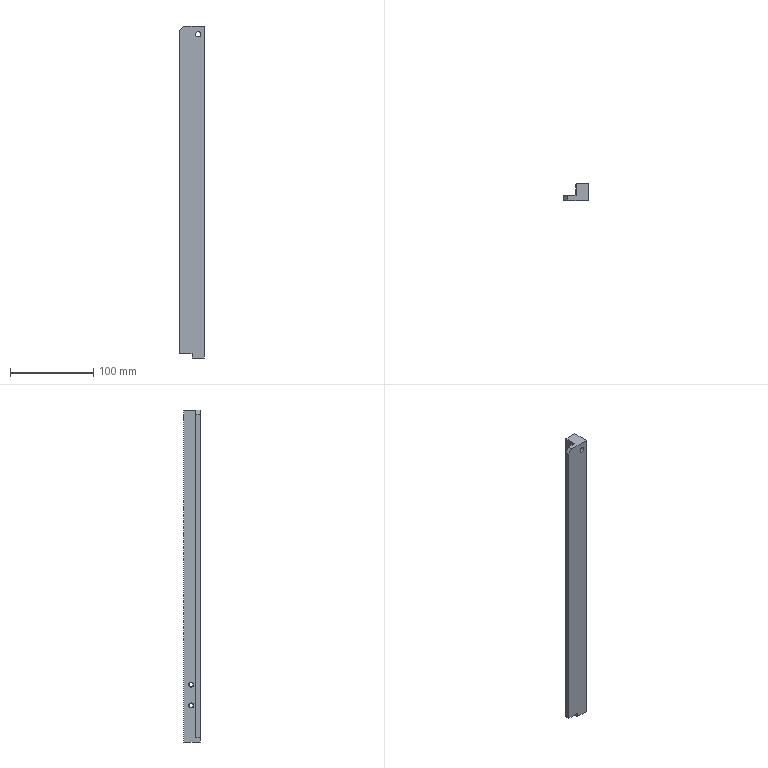Part | STEP file | Tube necking machine_id654_x_t | 1 solid | 17 faces | box 30 x 20 x 400 mm | volume 151258 mm3 | plane 10 | cone 4 | cylinder 3 | commonest cylinder face diameters 5 x2 6.5 x1
STEP:
#1=CARTESIAN_POINT('',(0.,0.,0.));
#2=DIRECTION('',(0.,0.,1.));
#3=DIRECTION('',(1.,0.,0.));
#4=AXIS2_PLACEMENT_3D('',#1,#2,#3);
#5=CARTESIAN_POINT('',(112.5,-108.,191.));
#6=VERTEX_POINT('',#5);
#7=CARTESIAN_POINT('',(97.5,-108.,191.));
#8=VERTEX_POINT('',#7);
#9=CARTESIAN_POINT('',(-10.,-108.,191.));
#10=DIRECTION('',(-1.,0.,0.));
#11=VECTOR('',#10,1.);
#12=LINE('',#9,#11);
#13=CARTESIAN_POINT('',(-10.,0.,191.));
#14=DIRECTION('',(0.,0.,1.));
#15=DIRECTION('',(-1.,0.,0.));
#16=AXIS2_PLACEMENT_3D('',#13,#14,#15);
#17=PLANE('',#16);
#18=CARTESIAN_POINT('',(0.,108.));
#19=DIRECTION('',(1.,0.));
#20=VECTOR('',#19,1.);
#21=LINE('',#18,#20);
#22=(GEOMETRIC_REPRESENTATION_CONTEXT(2)PARAMETRIC_REPRESENTATION_CONTEXT()REPRESENTATION_CONTEXT('',''));
#23=DEFINITIONAL_REPRESENTATION('',(#21),#22);
#24=PCURVE('',#17,#23);
#25=CARTESIAN_POINT('',(93.496,-108.,597.));
#26=DIRECTION('',(0.,1.,0.));
#27=DIRECTION('',(-1.,0.,0.));
#28=AXIS2_PLACEMENT_3D('',#25,#26,#27);
#29=PLANE('',#28);
#30=CARTESIAN_POINT('',(103.496,-406.));
#31=DIRECTION('',(1.,0.));
#32=VECTOR('',#31,1.);
#33=LINE('',#30,#32);
#34=(GEOMETRIC_REPRESENTATION_CONTEXT(2)PARAMETRIC_REPRESENTATION_CONTEXT()REPRESENTATION_CONTEXT('',''));
#35=DEFINITIONAL_REPRESENTATION('',(#33),#34);
#36=PCURVE('',#29,#35);
#37=SURFACE_CURVE('',#12,(#24,#36),.PCURVE_S1.);
#38=EDGE_CURVE('',#6,#8,#37,.T.);
#39=ORIENTED_EDGE('',*,*,#38,.F.);
#40=CARTESIAN_POINT('',(112.5,-128.,191.));
#41=VERTEX_POINT('',#40);
#42=CARTESIAN_POINT('',(112.5,-76.,191.));
#43=DIRECTION('',(0.,1.,0.));
#44=VECTOR('',#43,1.);
#45=LINE('',#42,#44);
#46=CARTESIAN_POINT('',(-122.5,76.));
#47=DIRECTION('',(0.,-1.));
#48=VECTOR('',#47,1.);
#49=LINE('',#46,#48);
#50=(GEOMETRIC_REPRESENTATION_CONTEXT(2)PARAMETRIC_REPRESENTATION_CONTEXT()REPRESENTATION_CONTEXT('',''));
#51=DEFINITIONAL_REPRESENTATION('',(#49),#50);
#52=PCURVE('',#17,#51);
#53=CARTESIAN_POINT('',(112.5,-76.,191.));
#54=DIRECTION('',(1.,0.,0.));
#55=DIRECTION('',(0.,-1.,0.));
#56=AXIS2_PLACEMENT_3D('',#53,#54,#55);
#57=PLANE('',#56);
#58=CARTESIAN_POINT('',(0.,0.));
#59=DIRECTION('',(-1.,0.));
#60=VECTOR('',#59,1.);
#61=LINE('',#58,#60);
#62=(GEOMETRIC_REPRESENTATION_CONTEXT(2)PARAMETRIC_REPRESENTATION_CONTEXT()REPRESENTATION_CONTEXT('',''));
#63=DEFINITIONAL_REPRESENTATION('',(#61),#62);
#64=PCURVE('',#57,#63);
#65=SURFACE_CURVE('',#45,(#52,#64),.PCURVE_S1.);
#66=EDGE_CURVE('',#41,#6,#65,.T.);
#67=ORIENTED_EDGE('',*,*,#66,.F.);
#68=CARTESIAN_POINT('',(97.5,-128.,191.));
#69=VERTEX_POINT('',#68);
#70=CARTESIAN_POINT('',(112.5,-128.,191.));
#71=DIRECTION('',(1.,0.,0.));
#72=VECTOR('',#71,1.);
#73=LINE('',#70,#72);
#74=CARTESIAN_POINT('',(-122.5,128.));
#75=DIRECTION('',(-1.,0.));
#76=VECTOR('',#75,1.);
#77=LINE('',#74,#76);
#78=(GEOMETRIC_REPRESENTATION_CONTEXT(2)PARAMETRIC_REPRESENTATION_CONTEXT()REPRESENTATION_CONTEXT('',''));
#79=DEFINITIONAL_REPRESENTATION('',(#77),#78);
#80=PCURVE('',#17,#79);
#81=CARTESIAN_POINT('',(112.5,-128.,191.));
#82=DIRECTION('',(0.,-1.,0.));
#83=DIRECTION('',(0.,0.,-1.));
#84=AXIS2_PLACEMENT_3D('',#81,#82,#83);
#85=PLANE('',#84);
#86=CARTESIAN_POINT('',(0.,0.));
#87=DIRECTION('',(0.,1.));
#88=VECTOR('',#87,1.);
#89=LINE('',#86,#88);
#90=(GEOMETRIC_REPRESENTATION_CONTEXT(2)PARAMETRIC_REPRESENTATION_CONTEXT()REPRESENTATION_CONTEXT('',''));
#91=DEFINITIONAL_REPRESENTATION('',(#89),#90);
#92=PCURVE('',#85,#91);
#93=SURFACE_CURVE('',#73,(#80,#92),.PCURVE_S1.);
#94=EDGE_CURVE('',#69,#41,#93,.T.);
#95=ORIENTED_EDGE('',*,*,#94,.F.);
#96=CARTESIAN_POINT('',(97.5,-124.5,191.));
#97=DIRECTION('',(0.,-1.,0.));
#98=VECTOR('',#97,1.);
#99=LINE('',#96,#98);
#100=CARTESIAN_POINT('',(-107.5,124.5));
#101=DIRECTION('',(0.,1.));
#102=VECTOR('',#101,1.);
#103=LINE('',#100,#102);
#104=(GEOMETRIC_REPRESENTATION_CONTEXT(2)PARAMETRIC_REPRESENTATION_CONTEXT()REPRESENTATION_CONTEXT('',''));
#105=DEFINITIONAL_REPRESENTATION('',(#103),#104);
#106=PCURVE('',#17,#105);
#107=CARTESIAN_POINT('',(97.5,-124.5,191.));
#108=DIRECTION('',(-1.,0.,0.));
#109=DIRECTION('',(0.,0.,-1.));
#110=AXIS2_PLACEMENT_3D('',#107,#108,#109);
#111=PLANE('',#110);
#112=CARTESIAN_POINT('',(0.,0.));
#113=DIRECTION('',(0.,1.));
#114=VECTOR('',#113,1.);
#115=LINE('',#112,#114);
#116=(GEOMETRIC_REPRESENTATION_CONTEXT(2)PARAMETRIC_REPRESENTATION_CONTEXT()REPRESENTATION_CONTEXT('',''));
#117=DEFINITIONAL_REPRESENTATION('',(#115),#116);
#118=PCURVE('',#111,#117);
#119=SURFACE_CURVE('',#99,(#106,#118),.PCURVE_S1.);
#120=EDGE_CURVE('',#8,#69,#119,.T.);
#121=ORIENTED_EDGE('',*,*,#120,.F.);
#122=EDGE_LOOP('',(#39,#67,#95,#121));
#123=FACE_BOUND('',#122,.T.);
#124=ADVANCED_FACE('',(#123),#17,.F.);
#125=CARTESIAN_POINT('',(112.5,-114.,235.));
#126=VERTEX_POINT('',#125);
#127=CARTESIAN_POINT('',(112.5,-117.,232.));
#128=VERTEX_POINT('',#127);
#129=CARTESIAN_POINT('',(112.5,-117.,235.));
#130=DIRECTION('',(-1.,0.,0.));
#131=DIRECTION('',(0.,1.,0.));
#132=AXIS2_PLACEMENT_3D('',#129,#130,#131);
#133=CIRCLE('',#132,3.);
#134=CARTESIAN_POINT('',(38.,-44.));
#135=CARTESIAN_POINT('',(38.,-38.804));
#136=CARTESIAN_POINT('',(42.5,-41.402));
#137=CARTESIAN_POINT('',(47.,-44.));
#138=CARTESIAN_POINT('',(42.5,-46.598));
#139=CARTESIAN_POINT('',(38.,-49.196));
#140=CARTESIAN_POINT('',(38.,-44.));
#141=(BOUNDED_CURVE()B_SPLINE_CURVE(2,(#134,#135,#136,#137,#138,#139,#140),.UNSPECIFIED.,.T.,.F.)B_SPLINE_CURVE_WITH_KNOTS((1,2,2,2,2,1),(-2.094,0.,2.094,4.189,6.283,8.378),.UNSPECIFIED.)CURVE()GEOMETRIC_REPRESENTATION_ITEM()RATIONAL_B_SPLINE_CURVE((1.,0.5,1.,0.5,1.,0.5,1.))REPRESENTATION_ITEM(''));
#142=(GEOMETRIC_REPRESENTATION_CONTEXT(2)PARAMETRIC_REPRESENTATION_CONTEXT()REPRESENTATION_CONTEXT('',''));
#143=DEFINITIONAL_REPRESENTATION('',(#141),#142);
#144=PCURVE('',#57,#143);
#145=CARTESIAN_POINT('',(112.5,-117.,235.));
#146=DIRECTION('',(1.,0.,0.));
#147=DIRECTION('',(0.,0.,-1.));
#148=AXIS2_PLACEMENT_3D('',#145,#146,#147);
#149=CONICAL_SURFACE('',#148,3.,0.7854);
#150=CARTESIAN_POINT('',(1.571,0.));
#151=DIRECTION('',(-1.,0.));
#152=VECTOR('',#151,1.);
#153=LINE('',#150,#152);
#154=(GEOMETRIC_REPRESENTATION_CONTEXT(2)PARAMETRIC_REPRESENTATION_CONTEXT()REPRESENTATION_CONTEXT('',''));
#155=DEFINITIONAL_REPRESENTATION('',(#153),#154);
#156=PCURVE('',#149,#155);
#157=SURFACE_CURVE('',#133,(#144,#156),.PCURVE_S1.);
#158=EDGE_CURVE('',#126,#128,#157,.T.);
#159=ORIENTED_EDGE('',*,*,#158,.T.);
#160=CARTESIAN_POINT('',(112.5,-117.,235.));
#161=DIRECTION('',(-1.,0.,0.));
#162=DIRECTION('',(0.,1.,0.));
#163=AXIS2_PLACEMENT_3D('',#160,#161,#162);
#164=CIRCLE('',#163,3.);
#165=CARTESIAN_POINT('',(38.,-44.));
#166=CARTESIAN_POINT('',(38.,-38.804));
#167=CARTESIAN_POINT('',(42.5,-41.402));
#168=CARTESIAN_POINT('',(47.,-44.));
#169=CARTESIAN_POINT('',(42.5,-46.598));
#170=CARTESIAN_POINT('',(38.,-49.196));
#171=CARTESIAN_POINT('',(38.,-44.));
#172=(BOUNDED_CURVE()B_SPLINE_CURVE(2,(#165,#166,#167,#168,#169,#170,#171),.UNSPECIFIED.,.T.,.F.)B_SPLINE_CURVE_WITH_KNOTS((1,2,2,2,2,1),(-2.094,0.,2.094,4.189,6.283,8.378),.UNSPECIFIED.)CURVE()GEOMETRIC_REPRESENTATION_ITEM()RATIONAL_B_SPLINE_CURVE((1.,0.5,1.,0.5,1.,0.5,1.))REPRESENTATION_ITEM(''));
#173=(GEOMETRIC_REPRESENTATION_CONTEXT(2)PARAMETRIC_REPRESENTATION_CONTEXT()REPRESENTATION_CONTEXT('',''));
#174=DEFINITIONAL_REPRESENTATION('',(#172),#173);
#175=PCURVE('',#57,#174);
#176=CARTESIAN_POINT('',(7.854,0.));
#177=DIRECTION('',(-1.,0.));
#178=VECTOR('',#177,1.);
#179=LINE('',#176,#178);
#180=(GEOMETRIC_REPRESENTATION_CONTEXT(2)PARAMETRIC_REPRESENTATION_CONTEXT()REPRESENTATION_CONTEXT('',''));
#181=DEFINITIONAL_REPRESENTATION('',(#179),#180);
#182=PCURVE('',#149,#181);
#183=SURFACE_CURVE('',#164,(#175,#182),.PCURVE_S1.);
#184=EDGE_CURVE('',#128,#126,#183,.T.);
#185=ORIENTED_EDGE('',*,*,#184,.T.);
#186=EDGE_LOOP('',(#159,#185));
#187=FACE_BOUND('',#186,.T.);
#188=CARTESIAN_POINT('',(112.5,-114.,260.));
#189=VERTEX_POINT('',#188);
#190=CARTESIAN_POINT('',(112.5,-117.,257.));
#191=VERTEX_POINT('',#190);
#192=CARTESIAN_POINT('',(112.5,-117.,260.));
#193=DIRECTION('',(-1.,0.,0.));
#194=DIRECTION('',(0.,1.,0.));
#195=AXIS2_PLACEMENT_3D('',#192,#193,#194);
#196=CIRCLE('',#195,3.);
#197=CARTESIAN_POINT('',(38.,-69.));
#198=CARTESIAN_POINT('',(38.,-63.804));
#199=CARTESIAN_POINT('',(42.5,-66.402));
#200=CARTESIAN_POINT('',(47.,-69.));
#201=CARTESIAN_POINT('',(42.5,-71.598));
#202=CARTESIAN_POINT('',(38.,-74.196));
#203=CARTESIAN_POINT('',(38.,-69.));
#204=(BOUNDED_CURVE()B_SPLINE_CURVE(2,(#197,#198,#199,#200,#201,#202,#203),.UNSPECIFIED.,.T.,.F.)B_SPLINE_CURVE_WITH_KNOTS((1,2,2,2,2,1),(-2.094,0.,2.094,4.189,6.283,8.378),.UNSPECIFIED.)CURVE()GEOMETRIC_REPRESENTATION_ITEM()RATIONAL_B_SPLINE_CURVE((1.,0.5,1.,0.5,1.,0.5,1.))REPRESENTATION_ITEM(''));
#205=(GEOMETRIC_REPRESENTATION_CONTEXT(2)PARAMETRIC_REPRESENTATION_CONTEXT()REPRESENTATION_CONTEXT('',''));
#206=DEFINITIONAL_REPRESENTATION('',(#204),#205);
#207=PCURVE('',#57,#206);
#208=CARTESIAN_POINT('',(112.5,-117.,260.));
#209=DIRECTION('',(1.,0.,0.));
#210=DIRECTION('',(0.,0.,-1.));
#211=AXIS2_PLACEMENT_3D('',#208,#209,#210);
#212=CONICAL_SURFACE('',#211,3.,0.7854);
#213=CARTESIAN_POINT('',(1.571,0.));
#214=DIRECTION('',(-1.,0.));
#215=VECTOR('',#214,1.);
#216=LINE('',#213,#215);
#217=(GEOMETRIC_REPRESENTATION_CONTEXT(2)PARAMETRIC_REPRESENTATION_CONTEXT()REPRESENTATION_CONTEXT('',''));
#218=DEFINITIONAL_REPRESENTATION('',(#216),#217);
#219=PCURVE('',#212,#218);
#220=SURFACE_CURVE('',#196,(#207,#219),.PCURVE_S1.);
#221=EDGE_CURVE('',#189,#191,#220,.T.);
#222=ORIENTED_EDGE('',*,*,#221,.T.);
#223=CARTESIAN_POINT('',(112.5,-117.,260.));
#224=DIRECTION('',(-1.,0.,0.));
#225=DIRECTION('',(0.,1.,0.));
#226=AXIS2_PLACEMENT_3D('',#223,#224,#225);
#227=CIRCLE('',#226,3.);
#228=CARTESIAN_POINT('',(38.,-69.));
#229=CARTESIAN_POINT('',(38.,-63.804));
#230=CARTESIAN_POINT('',(42.5,-66.402));
#231=CARTESIAN_POINT('',(47.,-69.));
#232=CARTESIAN_POINT('',(42.5,-71.598));
#233=CARTESIAN_POINT('',(38.,-74.196));
#234=CARTESIAN_POINT('',(38.,-69.));
#235=(BOUNDED_CURVE()B_SPLINE_CURVE(2,(#228,#229,#230,#231,#232,#233,#234),.UNSPECIFIED.,.T.,.F.)B_SPLINE_CURVE_WITH_KNOTS((1,2,2,2,2,1),(-2.094,0.,2.094,4.189,6.283,8.378),.UNSPECIFIED.)CURVE()GEOMETRIC_REPRESENTATION_ITEM()RATIONAL_B_SPLINE_CURVE((1.,0.5,1.,0.5,1.,0.5,1.))REPRESENTATION_ITEM(''));
#236=(GEOMETRIC_REPRESENTATION_CONTEXT(2)PARAMETRIC_REPRESENTATION_CONTEXT()REPRESENTATION_CONTEXT('',''));
#237=DEFINITIONAL_REPRESENTATION('',(#235),#236);
#238=PCURVE('',#57,#237);
#239=CARTESIAN_POINT('',(7.854,0.));
#240=DIRECTION('',(-1.,0.));
#241=VECTOR('',#240,1.);
#242=LINE('',#239,#241);
#243=(GEOMETRIC_REPRESENTATION_CONTEXT(2)PARAMETRIC_REPRESENTATION_CONTEXT()REPRESENTATION_CONTEXT('',''));
#244=DEFINITIONAL_REPRESENTATION('',(#242),#243);
#245=PCURVE('',#212,#244);
#246=SURFACE_CURVE('',#227,(#238,#245),.PCURVE_S1.);
#247=EDGE_CURVE('',#191,#189,#246,.T.);
#248=ORIENTED_EDGE('',*,*,#247,.T.);
#249=EDGE_LOOP('',(#222,#248));
#250=FACE_BOUND('',#249,.T.);
#251=ORIENTED_EDGE('',*,*,#66,.T.);
#252=CARTESIAN_POINT('',(112.5,-108.,591.));
#253=VERTEX_POINT('',#252);
#254=CARTESIAN_POINT('',(112.5,-108.,191.));
#255=DIRECTION('',(0.,0.,1.));
#256=VECTOR('',#255,1.);
#257=LINE('',#254,#256);
#258=CARTESIAN_POINT('',(32.,0.));
#259=DIRECTION('',(0.,-1.));
#260=VECTOR('',#259,1.);
#261=LINE('',#258,#260);
#262=(GEOMETRIC_REPRESENTATION_CONTEXT(2)PARAMETRIC_REPRESENTATION_CONTEXT()REPRESENTATION_CONTEXT('',''));
#263=DEFINITIONAL_REPRESENTATION('',(#261),#262);
#264=PCURVE('',#57,#263);
#265=CARTESIAN_POINT('',(-19.004,-406.));
#266=DIRECTION('',(0.,1.));
#267=VECTOR('',#266,1.);
#268=LINE('',#265,#267);
#269=(GEOMETRIC_REPRESENTATION_CONTEXT(2)PARAMETRIC_REPRESENTATION_CONTEXT()REPRESENTATION_CONTEXT('',''));
#270=DEFINITIONAL_REPRESENTATION('',(#268),#269);
#271=PCURVE('',#29,#270);
#272=SURFACE_CURVE('',#257,(#264,#271),.PCURVE_S1.);
#273=EDGE_CURVE('',#6,#253,#272,.T.);
#274=ORIENTED_EDGE('',*,*,#273,.T.);
#275=CARTESIAN_POINT('',(112.5,-128.,591.));
#276=VERTEX_POINT('',#275);
#277=CARTESIAN_POINT('',(112.5,-76.,591.));
#278=DIRECTION('',(0.,1.,0.));
#279=VECTOR('',#278,1.);
#280=LINE('',#277,#279);
#281=CARTESIAN_POINT('',(0.,-400.));
#282=DIRECTION('',(-1.,0.));
#283=VECTOR('',#282,1.);
#284=LINE('',#281,#283);
#285=(GEOMETRIC_REPRESENTATION_CONTEXT(2)PARAMETRIC_REPRESENTATION_CONTEXT()REPRESENTATION_CONTEXT('',''));
#286=DEFINITIONAL_REPRESENTATION('',(#284),#285);
#287=PCURVE('',#57,#286);
#288=CARTESIAN_POINT('',(-10.,0.,591.));
#289=DIRECTION('',(0.,0.,1.));
#290=DIRECTION('',(-1.,0.,0.));
#291=AXIS2_PLACEMENT_3D('',#288,#289,#290);
#292=PLANE('',#291);
#293=CARTESIAN_POINT('',(-122.5,76.));
#294=DIRECTION('',(0.,-1.));
#295=VECTOR('',#294,1.);
#296=LINE('',#293,#295);
#297=(GEOMETRIC_REPRESENTATION_CONTEXT(2)PARAMETRIC_REPRESENTATION_CONTEXT()REPRESENTATION_CONTEXT('',''));
#298=DEFINITIONAL_REPRESENTATION('',(#296),#297);
#299=PCURVE('',#292,#298);
#300=SURFACE_CURVE('',#280,(#287,#299),.PCURVE_S1.);
#301=EDGE_CURVE('',#276,#253,#300,.T.);
#302=ORIENTED_EDGE('',*,*,#301,.F.);
#303=CARTESIAN_POINT('',(112.5,-128.,191.));
#304=DIRECTION('',(0.,0.,-1.));
#305=VECTOR('',#304,1.);
#306=LINE('',#303,#305);
#307=CARTESIAN_POINT('',(52.,0.));
#308=DIRECTION('',(0.,1.));
#309=VECTOR('',#308,1.);
#310=LINE('',#307,#309);
#311=(GEOMETRIC_REPRESENTATION_CONTEXT(2)PARAMETRIC_REPRESENTATION_CONTEXT()REPRESENTATION_CONTEXT('',''));
#312=DEFINITIONAL_REPRESENTATION('',(#310),#311);
#313=PCURVE('',#57,#312);
#314=CARTESIAN_POINT('',(0.,0.));
#315=DIRECTION('',(1.,0.));
#316=VECTOR('',#315,1.);
#317=LINE('',#314,#316);
#318=(GEOMETRIC_REPRESENTATION_CONTEXT(2)PARAMETRIC_REPRESENTATION_CONTEXT()REPRESENTATION_CONTEXT('',''));
#319=DEFINITIONAL_REPRESENTATION('',(#317),#318);
#320=PCURVE('',#85,#319);
#321=SURFACE_CURVE('',#306,(#313,#320),.PCURVE_S1.);
#322=EDGE_CURVE('',#276,#41,#321,.T.);
#323=ORIENTED_EDGE('',*,*,#322,.T.);
#324=EDGE_LOOP('',(#251,#274,#302,#323));
#325=FACE_BOUND('',#324,.T.);
#326=ADVANCED_FACE('',(#187,#250,#325),#57,.T.);
#327=CARTESIAN_POINT('',(97.5,-120.,235.));
#328=VERTEX_POINT('',#327);
#329=CARTESIAN_POINT('',(97.5,-117.,238.));
#330=VERTEX_POINT('',#329);
#331=CARTESIAN_POINT('',(97.5,-117.,235.));
#332=DIRECTION('',(1.,0.,0.));
#333=DIRECTION('',(0.,-1.,0.));
#334=AXIS2_PLACEMENT_3D('',#331,#332,#333);
#335=CIRCLE('',#334,3.);
#336=CARTESIAN_POINT('',(-44.,-4.5));
#337=CARTESIAN_POINT('',(-38.804,-4.5));
#338=CARTESIAN_POINT('',(-41.402,-9.));
#339=CARTESIAN_POINT('',(-44.,-13.5));
#340=CARTESIAN_POINT('',(-46.598,-9.));
#341=CARTESIAN_POINT('',(-49.196,-4.5));
#342=CARTESIAN_POINT('',(-44.,-4.5));
#343=(BOUNDED_CURVE()B_SPLINE_CURVE(2,(#336,#337,#338,#339,#340,#341,#342),.UNSPECIFIED.,.T.,.F.)B_SPLINE_CURVE_WITH_KNOTS((1,2,2,2,2,1),(-2.094,0.,2.094,4.189,6.283,8.378),.UNSPECIFIED.)CURVE()GEOMETRIC_REPRESENTATION_ITEM()RATIONAL_B_SPLINE_CURVE((1.,0.5,1.,0.5,1.,0.5,1.))REPRESENTATION_ITEM(''));
#344=(GEOMETRIC_REPRESENTATION_CONTEXT(2)PARAMETRIC_REPRESENTATION_CONTEXT()REPRESENTATION_CONTEXT('',''));
#345=DEFINITIONAL_REPRESENTATION('',(#343),#344);
#346=PCURVE('',#111,#345);
#347=CARTESIAN_POINT('',(98.,-117.,235.));
#348=DIRECTION('',(-1.,0.,0.));
#349=DIRECTION('',(0.,0.,1.));
#350=AXIS2_PLACEMENT_3D('',#347,#348,#349);
#351=CONICAL_SURFACE('',#350,2.5,0.7854);
#352=CARTESIAN_POINT('',(4.712,0.5));
#353=DIRECTION('',(-1.,0.));
#354=VECTOR('',#353,1.);
#355=LINE('',#352,#354);
#356=(GEOMETRIC_REPRESENTATION_CONTEXT(2)PARAMETRIC_REPRESENTATION_CONTEXT()REPRESENTATION_CONTEXT('',''));
#357=DEFINITIONAL_REPRESENTATION('',(#355),#356);
#358=PCURVE('',#351,#357);
#359=SURFACE_CURVE('',#335,(#346,#358),.PCURVE_S1.);
#360=EDGE_CURVE('',#328,#330,#359,.T.);
#361=ORIENTED_EDGE('',*,*,#360,.T.);
#362=CARTESIAN_POINT('',(97.5,-117.,235.));
#363=DIRECTION('',(1.,0.,0.));
#364=DIRECTION('',(0.,-1.,0.));
#365=AXIS2_PLACEMENT_3D('',#362,#363,#364);
#366=CIRCLE('',#365,3.);
#367=CARTESIAN_POINT('',(-44.,-4.5));
#368=CARTESIAN_POINT('',(-38.804,-4.5));
#369=CARTESIAN_POINT('',(-41.402,-9.));
#370=CARTESIAN_POINT('',(-44.,-13.5));
#371=CARTESIAN_POINT('',(-46.598,-9.));
#372=CARTESIAN_POINT('',(-49.196,-4.5));
#373=CARTESIAN_POINT('',(-44.,-4.5));
#374=(BOUNDED_CURVE()B_SPLINE_CURVE(2,(#367,#368,#369,#370,#371,#372,#373),.UNSPECIFIED.,.T.,.F.)B_SPLINE_CURVE_WITH_KNOTS((1,2,2,2,2,1),(-2.094,0.,2.094,4.189,6.283,8.378),.UNSPECIFIED.)CURVE()GEOMETRIC_REPRESENTATION_ITEM()RATIONAL_B_SPLINE_CURVE((1.,0.5,1.,0.5,1.,0.5,1.))REPRESENTATION_ITEM(''));
#375=(GEOMETRIC_REPRESENTATION_CONTEXT(2)PARAMETRIC_REPRESENTATION_CONTEXT()REPRESENTATION_CONTEXT('',''));
#376=DEFINITIONAL_REPRESENTATION('',(#374),#375);
#377=PCURVE('',#111,#376);
#378=CARTESIAN_POINT('',(10.996,0.5));
#379=DIRECTION('',(-1.,0.));
#380=VECTOR('',#379,1.);
#381=LINE('',#378,#380);
#382=(GEOMETRIC_REPRESENTATION_CONTEXT(2)PARAMETRIC_REPRESENTATION_CONTEXT()REPRESENTATION_CONTEXT('',''));
#383=DEFINITIONAL_REPRESENTATION('',(#381),#382);
#384=PCURVE('',#351,#383);
#385=SURFACE_CURVE('',#366,(#377,#384),.PCURVE_S1.);
#386=EDGE_CURVE('',#330,#328,#385,.T.);
#387=ORIENTED_EDGE('',*,*,#386,.T.);
#388=EDGE_LOOP('',(#361,#387));
#389=FACE_BOUND('',#388,.T.);
#390=CARTESIAN_POINT('',(97.5,-120.,260.));
#391=VERTEX_POINT('',#390);
#392=CARTESIAN_POINT('',(97.5,-117.,263.));
#393=VERTEX_POINT('',#392);
#394=CARTESIAN_POINT('',(97.5,-117.,260.));
#395=DIRECTION('',(1.,0.,0.));
#396=DIRECTION('',(0.,-1.,0.));
#397=AXIS2_PLACEMENT_3D('',#394,#395,#396);
#398=CIRCLE('',#397,3.);
#399=CARTESIAN_POINT('',(-69.,-4.5));
#400=CARTESIAN_POINT('',(-63.804,-4.5));
#401=CARTESIAN_POINT('',(-66.402,-9.));
#402=CARTESIAN_POINT('',(-69.,-13.5));
#403=CARTESIAN_POINT('',(-71.598,-9.));
#404=CARTESIAN_POINT('',(-74.196,-4.5));
#405=CARTESIAN_POINT('',(-69.,-4.5));
#406=(BOUNDED_CURVE()B_SPLINE_CURVE(2,(#399,#400,#401,#402,#403,#404,#405),.UNSPECIFIED.,.T.,.F.)B_SPLINE_CURVE_WITH_KNOTS((1,2,2,2,2,1),(-2.094,0.,2.094,4.189,6.283,8.378),.UNSPECIFIED.)CURVE()GEOMETRIC_REPRESENTATION_ITEM()RATIONAL_B_SPLINE_CURVE((1.,0.5,1.,0.5,1.,0.5,1.))REPRESENTATION_ITEM(''));
#407=(GEOMETRIC_REPRESENTATION_CONTEXT(2)PARAMETRIC_REPRESENTATION_CONTEXT()REPRESENTATION_CONTEXT('',''));
#408=DEFINITIONAL_REPRESENTATION('',(#406),#407);
#409=PCURVE('',#111,#408);
#410=CARTESIAN_POINT('',(98.,-117.,260.));
#411=DIRECTION('',(-1.,0.,0.));
#412=DIRECTION('',(0.,0.,1.));
#413=AXIS2_PLACEMENT_3D('',#410,#411,#412);
#414=CONICAL_SURFACE('',#413,2.5,0.7854);
#415=CARTESIAN_POINT('',(4.712,0.5));
#416=DIRECTION('',(-1.,0.));
#417=VECTOR('',#416,1.);
#418=LINE('',#415,#417);
#419=(GEOMETRIC_REPRESENTATION_CONTEXT(2)PARAMETRIC_REPRESENTATION_CONTEXT()REPRESENTATION_CONTEXT('',''));
#420=DEFINITIONAL_REPRESENTATION('',(#418),#419);
#421=PCURVE('',#414,#420);
#422=SURFACE_CURVE('',#398,(#409,#421),.PCURVE_S1.);
#423=EDGE_CURVE('',#391,#393,#422,.T.);
#424=ORIENTED_EDGE('',*,*,#423,.T.);
#425=CARTESIAN_POINT('',(97.5,-117.,260.));
#426=DIRECTION('',(1.,0.,0.));
#427=DIRECTION('',(0.,-1.,0.));
#428=AXIS2_PLACEMENT_3D('',#425,#426,#427);
#429=CIRCLE('',#428,3.);
#430=CARTESIAN_POINT('',(-69.,-4.5));
#431=CARTESIAN_POINT('',(-63.804,-4.5));
#432=CARTESIAN_POINT('',(-66.402,-9.));
#433=CARTESIAN_POINT('',(-69.,-13.5));
#434=CARTESIAN_POINT('',(-71.598,-9.));
#435=CARTESIAN_POINT('',(-74.196,-4.5));
#436=CARTESIAN_POINT('',(-69.,-4.5));
#437=(BOUNDED_CURVE()B_SPLINE_CURVE(2,(#430,#431,#432,#433,#434,#435,#436),.UNSPECIFIED.,.T.,.F.)B_SPLINE_CURVE_WITH_KNOTS((1,2,2,2,2,1),(-2.094,0.,2.094,4.189,6.283,8.378),.UNSPECIFIED.)CURVE()GEOMETRIC_REPRESENTATION_ITEM()RATIONAL_B_SPLINE_CURVE((1.,0.5,1.,0.5,1.,0.5,1.))REPRESENTATION_ITEM(''));
#438=(GEOMETRIC_REPRESENTATION_CONTEXT(2)PARAMETRIC_REPRESENTATION_CONTEXT()REPRESENTATION_CONTEXT('',''));
#439=DEFINITIONAL_REPRESENTATION('',(#437),#438);
#440=PCURVE('',#111,#439);
#441=CARTESIAN_POINT('',(10.996,0.5));
#442=DIRECTION('',(-1.,0.));
#443=VECTOR('',#442,1.);
#444=LINE('',#441,#443);
#445=(GEOMETRIC_REPRESENTATION_CONTEXT(2)PARAMETRIC_REPRESENTATION_CONTEXT()REPRESENTATION_CONTEXT('',''));
#446=DEFINITIONAL_REPRESENTATION('',(#444),#445);
#447=PCURVE('',#414,#446);
#448=SURFACE_CURVE('',#429,(#440,#447),.PCURVE_S1.);
#449=EDGE_CURVE('',#393,#391,#448,.T.);
#450=ORIENTED_EDGE('',*,*,#449,.T.);
#451=EDGE_LOOP('',(#424,#450));
#452=FACE_BOUND('',#451,.T.);
#453=CARTESIAN_POINT('',(97.5,-108.,591.));
#454=VERTEX_POINT('',#453);
#455=CARTESIAN_POINT('',(97.5,-122.5,591.));
#456=VERTEX_POINT('',#455);
#457=CARTESIAN_POINT('',(97.5,-124.5,591.));
#458=DIRECTION('',(0.,-1.,0.));
#459=VECTOR('',#458,1.);
#460=LINE('',#457,#459);
#461=CARTESIAN_POINT('',(-400.,0.));
#462=DIRECTION('',(0.,1.));
#463=VECTOR('',#462,1.);
#464=LINE('',#461,#463);
#465=(GEOMETRIC_REPRESENTATION_CONTEXT(2)PARAMETRIC_REPRESENTATION_CONTEXT()REPRESENTATION_CONTEXT('',''));
#466=DEFINITIONAL_REPRESENTATION('',(#464),#465);
#467=PCURVE('',#111,#466);
#468=CARTESIAN_POINT('',(-107.5,124.5));
#469=DIRECTION('',(0.,1.));
#470=VECTOR('',#469,1.);
#471=LINE('',#468,#470);
#472=(GEOMETRIC_REPRESENTATION_CONTEXT(2)PARAMETRIC_REPRESENTATION_CONTEXT()REPRESENTATION_CONTEXT('',''));
#473=DEFINITIONAL_REPRESENTATION('',(#471),#472);
#474=PCURVE('',#292,#473);
#475=SURFACE_CURVE('',#460,(#467,#474),.PCURVE_S1.);
#476=EDGE_CURVE('',#454,#456,#475,.T.);
#477=ORIENTED_EDGE('',*,*,#476,.F.);
#478=CARTESIAN_POINT('',(97.5,-108.,191.));
#479=DIRECTION('',(0.,0.,-1.));
#480=VECTOR('',#479,1.);
#481=LINE('',#478,#480);
#482=CARTESIAN_POINT('',(0.,-16.5));
#483=DIRECTION('',(1.,0.));
#484=VECTOR('',#483,1.);
#485=LINE('',#482,#484);
#486=(GEOMETRIC_REPRESENTATION_CONTEXT(2)PARAMETRIC_REPRESENTATION_CONTEXT()REPRESENTATION_CONTEXT('',''));
#487=DEFINITIONAL_REPRESENTATION('',(#485),#486);
#488=PCURVE('',#111,#487);
#489=CARTESIAN_POINT('',(-4.004,-406.));
#490=DIRECTION('',(0.,-1.));
#491=VECTOR('',#490,1.);
#492=LINE('',#489,#491);
#493=(GEOMETRIC_REPRESENTATION_CONTEXT(2)PARAMETRIC_REPRESENTATION_CONTEXT()REPRESENTATION_CONTEXT('',''));
#494=DEFINITIONAL_REPRESENTATION('',(#492),#493);
#495=PCURVE('',#29,#494);
#496=SURFACE_CURVE('',#481,(#488,#495),.PCURVE_S1.);
#497=EDGE_CURVE('',#454,#8,#496,.T.);
#498=ORIENTED_EDGE('',*,*,#497,.T.);
#499=ORIENTED_EDGE('',*,*,#120,.T.);
#500=CARTESIAN_POINT('',(97.5,-128.,196.));
#501=VERTEX_POINT('',#500);
#502=CARTESIAN_POINT('',(97.5,-128.,191.));
#503=DIRECTION('',(0.,0.,-1.));
#504=VECTOR('',#503,1.);
#505=LINE('',#502,#504);
#506=CARTESIAN_POINT('',(0.,3.5));
#507=DIRECTION('',(1.,0.));
#508=VECTOR('',#507,1.);
#509=LINE('',#506,#508);
#510=(GEOMETRIC_REPRESENTATION_CONTEXT(2)PARAMETRIC_REPRESENTATION_CONTEXT()REPRESENTATION_CONTEXT('',''));
#511=DEFINITIONAL_REPRESENTATION('',(#509),#510);
#512=PCURVE('',#111,#511);
#513=CARTESIAN_POINT('',(0.,-15.));
#514=DIRECTION('',(1.,0.));
#515=VECTOR('',#514,1.);
#516=LINE('',#513,#515);
#517=(GEOMETRIC_REPRESENTATION_CONTEXT(2)PARAMETRIC_REPRESENTATION_CONTEXT()REPRESENTATION_CONTEXT('',''));
#518=DEFINITIONAL_REPRESENTATION('',(#516),#517);
#519=PCURVE('',#85,#518);
#520=SURFACE_CURVE('',#505,(#512,#519),.PCURVE_S1.);
#521=EDGE_CURVE('',#501,#69,#520,.T.);
#522=ORIENTED_EDGE('',*,*,#521,.F.);
#523=CARTESIAN_POINT('',(97.5,-122.5,196.));
#524=VERTEX_POINT('',#523);
#525=CARTESIAN_POINT('',(97.5,-259.,196.));
#526=DIRECTION('',(0.,1.,0.));
#527=VECTOR('',#526,1.);
#528=LINE('',#525,#527);
#529=CARTESIAN_POINT('',(-5.,134.5));
#530=DIRECTION('',(0.,-1.));
#531=VECTOR('',#530,1.);
#532=LINE('',#529,#531);
#533=(GEOMETRIC_REPRESENTATION_CONTEXT(2)PARAMETRIC_REPRESENTATION_CONTEXT()REPRESENTATION_CONTEXT('',''));
#534=DEFINITIONAL_REPRESENTATION('',(#532),#533);
#535=PCURVE('',#111,#534);
#536=CARTESIAN_POINT('',(50.,-259.,196.));
#537=DIRECTION('',(0.,0.,-1.));
#538=DIRECTION('',(1.,0.,0.));
#539=AXIS2_PLACEMENT_3D('',#536,#537,#538);
#540=PLANE('',#539);
#541=CARTESIAN_POINT('',(47.5,0.));
#542=DIRECTION('',(0.,-1.));
#543=VECTOR('',#542,1.);
#544=LINE('',#541,#543);
#545=(GEOMETRIC_REPRESENTATION_CONTEXT(2)PARAMETRIC_REPRESENTATION_CONTEXT()REPRESENTATION_CONTEXT('',''));
#546=DEFINITIONAL_REPRESENTATION('',(#544),#545);
#547=PCURVE('',#540,#546);
#548=SURFACE_CURVE('',#528,(#535,#547),.PCURVE_S1.);
#549=EDGE_CURVE('',#501,#524,#548,.T.);
#550=ORIENTED_EDGE('',*,*,#549,.T.);
#551=CARTESIAN_POINT('',(97.5,-122.5,191.));
#552=DIRECTION('',(0.,0.,-1.));
#553=VECTOR('',#552,1.);
#554=LINE('',#551,#553);
#555=CARTESIAN_POINT('',(0.,-2.));
#556=DIRECTION('',(1.,0.));
#557=VECTOR('',#556,1.);
#558=LINE('',#555,#557);
#559=(GEOMETRIC_REPRESENTATION_CONTEXT(2)PARAMETRIC_REPRESENTATION_CONTEXT()REPRESENTATION_CONTEXT('',''));
#560=DEFINITIONAL_REPRESENTATION('',(#558),#559);
#561=PCURVE('',#111,#560);
#562=CARTESIAN_POINT('',(82.5,-122.5,191.));
#563=DIRECTION('',(0.,1.,0.));
#564=DIRECTION('',(0.,0.,1.));
#565=AXIS2_PLACEMENT_3D('',#562,#563,#564);
#566=PLANE('',#565);
#567=CARTESIAN_POINT('',(0.,15.));
#568=DIRECTION('',(-1.,0.));
#569=VECTOR('',#568,1.);
#570=LINE('',#567,#569);
#571=(GEOMETRIC_REPRESENTATION_CONTEXT(2)PARAMETRIC_REPRESENTATION_CONTEXT()REPRESENTATION_CONTEXT('',''));
#572=DEFINITIONAL_REPRESENTATION('',(#570),#571);
#573=PCURVE('',#566,#572);
#574=SURFACE_CURVE('',#554,(#561,#573),.PCURVE_S1.);
#575=EDGE_CURVE('',#456,#524,#574,.T.);
#576=ORIENTED_EDGE('',*,*,#575,.F.);
#577=EDGE_LOOP('',(#477,#498,#499,#522,#550,#576));
#578=FACE_BOUND('',#577,.T.);
#579=ADVANCED_FACE('',(#389,#452,#578),#111,.T.);
#580=CARTESIAN_POINT('',(87.5,-122.5,591.));
#581=VERTEX_POINT('',#580);
#582=CARTESIAN_POINT('',(-10.,-122.5,591.));
#583=DIRECTION('',(-1.,0.,0.));
#584=VECTOR('',#583,1.);
#585=LINE('',#582,#584);
#586=CARTESIAN_POINT('',(0.,122.5));
#587=DIRECTION('',(1.,0.));
#588=VECTOR('',#587,1.);
#589=LINE('',#586,#588);
#590=(GEOMETRIC_REPRESENTATION_CONTEXT(2)PARAMETRIC_REPRESENTATION_CONTEXT()REPRESENTATION_CONTEXT('',''));
#591=DEFINITIONAL_REPRESENTATION('',(#589),#590);
#592=PCURVE('',#292,#591);
#593=CARTESIAN_POINT('',(400.,-92.5));
#594=DIRECTION('',(0.,-1.));
#595=VECTOR('',#594,1.);
#596=LINE('',#593,#595);
#597=(GEOMETRIC_REPRESENTATION_CONTEXT(2)PARAMETRIC_REPRESENTATION_CONTEXT()REPRESENTATION_CONTEXT('',''));
#598=DEFINITIONAL_REPRESENTATION('',(#596),#597);
#599=PCURVE('',#566,#598);
#600=SURFACE_CURVE('',#585,(#592,#599),.PCURVE_S1.);
#601=EDGE_CURVE('',#456,#581,#600,.T.);
#602=ORIENTED_EDGE('',*,*,#601,.T.);
#603=CARTESIAN_POINT('',(87.5,-128.,591.));
#604=VERTEX_POINT('',#603);
#605=CARTESIAN_POINT('',(87.5,0.,591.));
#606=DIRECTION('',(0.,-1.,0.));
#607=VECTOR('',#606,1.);
#608=LINE('',#605,#607);
#609=CARTESIAN_POINT('',(-97.5,0.));
#610=DIRECTION('',(0.,1.));
#611=VECTOR('',#610,1.);
#612=LINE('',#609,#611);
#613=(GEOMETRIC_REPRESENTATION_CONTEXT(2)PARAMETRIC_REPRESENTATION_CONTEXT()REPRESENTATION_CONTEXT('',''));
#614=DEFINITIONAL_REPRESENTATION('',(#612),#613);
#615=PCURVE('',#292,#614);
#616=CARTESIAN_POINT('',(87.5,0.,591.));
#617=DIRECTION('',(0.7071,0.,-0.7071));
#618=DIRECTION('',(0.,-1.,0.));
#619=AXIS2_PLACEMENT_3D('',#616,#617,#618);
#620=PLANE('',#619);
#621=CARTESIAN_POINT('',(0.,0.));
#622=DIRECTION('',(1.,0.));
#623=VECTOR('',#622,1.);
#624=LINE('',#621,#623);
#625=(GEOMETRIC_REPRESENTATION_CONTEXT(2)PARAMETRIC_REPRESENTATION_CONTEXT()REPRESENTATION_CONTEXT('',''));
#626=DEFINITIONAL_REPRESENTATION('',(#624),#625);
#627=PCURVE('',#620,#626);
#628=SURFACE_CURVE('',#608,(#615,#627),.PCURVE_S1.);
#629=EDGE_CURVE('',#581,#604,#628,.T.);
#630=ORIENTED_EDGE('',*,*,#629,.T.);
#631=CARTESIAN_POINT('',(112.5,-128.,591.));
#632=DIRECTION('',(1.,0.,0.));
#633=VECTOR('',#632,1.);
#634=LINE('',#631,#633);
#635=CARTESIAN_POINT('',(-122.5,128.));
#636=DIRECTION('',(-1.,0.));
#637=VECTOR('',#636,1.);
#638=LINE('',#635,#637);
#639=(GEOMETRIC_REPRESENTATION_CONTEXT(2)PARAMETRIC_REPRESENTATION_CONTEXT()REPRESENTATION_CONTEXT('',''));
#640=DEFINITIONAL_REPRESENTATION('',(#638),#639);
#641=PCURVE('',#292,#640);
#642=CARTESIAN_POINT('',(-400.,0.));
#643=DIRECTION('',(0.,1.));
#644=VECTOR('',#643,1.);
#645=LINE('',#642,#644);
#646=(GEOMETRIC_REPRESENTATION_CONTEXT(2)PARAMETRIC_REPRESENTATION_CONTEXT()REPRESENTATION_CONTEXT('',''));
#647=DEFINITIONAL_REPRESENTATION('',(#645),#646);
#648=PCURVE('',#85,#647);
#649=SURFACE_CURVE('',#634,(#641,#648),.PCURVE_S1.);
#650=EDGE_CURVE('',#604,#276,#649,.T.);
#651=ORIENTED_EDGE('',*,*,#650,.T.);
#652=ORIENTED_EDGE('',*,*,#301,.T.);
#653=CARTESIAN_POINT('',(-10.,-108.,591.));
#654=DIRECTION('',(-1.,0.,0.));
#655=VECTOR('',#654,1.);
#656=LINE('',#653,#655);
#657=CARTESIAN_POINT('',(0.,108.));
#658=DIRECTION('',(1.,0.));
#659=VECTOR('',#658,1.);
#660=LINE('',#657,#659);
#661=(GEOMETRIC_REPRESENTATION_CONTEXT(2)PARAMETRIC_REPRESENTATION_CONTEXT()REPRESENTATION_CONTEXT('',''));
#662=DEFINITIONAL_REPRESENTATION('',(#660),#661);
#663=PCURVE('',#292,#662);
#664=CARTESIAN_POINT('',(103.496,-6.));
#665=DIRECTION('',(1.,0.));
#666=VECTOR('',#665,1.);
#667=LINE('',#664,#666);
#668=(GEOMETRIC_REPRESENTATION_CONTEXT(2)PARAMETRIC_REPRESENTATION_CONTEXT()REPRESENTATION_CONTEXT('',''));
#669=DEFINITIONAL_REPRESENTATION('',(#667),#668);
#670=PCURVE('',#29,#669);
#671=SURFACE_CURVE('',#656,(#663,#670),.PCURVE_S1.);
#672=EDGE_CURVE('',#253,#454,#671,.T.);
#673=ORIENTED_EDGE('',*,*,#672,.T.);
#674=ORIENTED_EDGE('',*,*,#476,.T.);
#675=EDGE_LOOP('',(#602,#630,#651,#652,#673,#674));
#676=FACE_BOUND('',#675,.T.);
#677=ADVANCED_FACE('',(#676),#292,.T.);
#678=CARTESIAN_POINT('',(82.5,-128.,586.));
#679=VERTEX_POINT('',#678);
#680=CARTESIAN_POINT('',(82.5,-128.,196.));
#681=VERTEX_POINT('',#680);
#682=CARTESIAN_POINT('',(82.5,-128.,191.));
#683=DIRECTION('',(0.,0.,-1.));
#684=VECTOR('',#683,1.);
#685=LINE('',#682,#684);
#686=CARTESIAN_POINT('',(82.5,-128.,191.));
#687=DIRECTION('',(-1.,0.,0.));
#688=DIRECTION('',(0.,0.,-1.));
#689=AXIS2_PLACEMENT_3D('',#686,#687,#688);
#690=PLANE('',#689);
#691=CARTESIAN_POINT('',(0.,0.));
#692=DIRECTION('',(1.,0.));
#693=VECTOR('',#692,1.);
#694=LINE('',#691,#693);
#695=(GEOMETRIC_REPRESENTATION_CONTEXT(2)PARAMETRIC_REPRESENTATION_CONTEXT()REPRESENTATION_CONTEXT('',''));
#696=DEFINITIONAL_REPRESENTATION('',(#694),#695);
#697=PCURVE('',#690,#696);
#698=CARTESIAN_POINT('',(0.,-30.));
#699=DIRECTION('',(1.,0.));
#700=VECTOR('',#699,1.);
#701=LINE('',#698,#700);
#702=(GEOMETRIC_REPRESENTATION_CONTEXT(2)PARAMETRIC_REPRESENTATION_CONTEXT()REPRESENTATION_CONTEXT('',''));
#703=DEFINITIONAL_REPRESENTATION('',(#701),#702);
#704=PCURVE('',#85,#703);
#705=SURFACE_CURVE('',#685,(#697,#704),.PCURVE_S1.);
#706=EDGE_CURVE('',#679,#681,#705,.T.);
#707=ORIENTED_EDGE('',*,*,#706,.F.);
#708=CARTESIAN_POINT('',(82.5,-122.5,586.));
#709=VERTEX_POINT('',#708);
#710=CARTESIAN_POINT('',(82.5,-128.,586.));
#711=DIRECTION('',(0.,1.,0.));
#712=VECTOR('',#711,1.);
#713=LINE('',#710,#712);
#714=CARTESIAN_POINT('',(-395.,0.));
#715=DIRECTION('',(0.,-1.));
#716=VECTOR('',#715,1.);
#717=LINE('',#714,#716);
#718=(GEOMETRIC_REPRESENTATION_CONTEXT(2)PARAMETRIC_REPRESENTATION_CONTEXT()REPRESENTATION_CONTEXT('',''));
#719=DEFINITIONAL_REPRESENTATION('',(#717),#718);
#720=PCURVE('',#690,#719);
#721=CARTESIAN_POINT('',(128.,7.071));
#722=DIRECTION('',(-1.,0.));
#723=VECTOR('',#722,1.);
#724=LINE('',#721,#723);
#725=(GEOMETRIC_REPRESENTATION_CONTEXT(2)PARAMETRIC_REPRESENTATION_CONTEXT()REPRESENTATION_CONTEXT('',''));
#726=DEFINITIONAL_REPRESENTATION('',(#724),#725);
#727=PCURVE('',#620,#726);
#728=SURFACE_CURVE('',#713,(#720,#727),.PCURVE_S1.);
#729=EDGE_CURVE('',#679,#709,#728,.T.);
#730=ORIENTED_EDGE('',*,*,#729,.T.);
#731=CARTESIAN_POINT('',(82.5,-122.5,196.));
#732=VERTEX_POINT('',#731);
#733=CARTESIAN_POINT('',(82.5,-122.5,191.));
#734=DIRECTION('',(0.,0.,-1.));
#735=VECTOR('',#734,1.);
#736=LINE('',#733,#735);
#737=CARTESIAN_POINT('',(0.,-5.5));
#738=DIRECTION('',(1.,0.));
#739=VECTOR('',#738,1.);
#740=LINE('',#737,#739);
#741=(GEOMETRIC_REPRESENTATION_CONTEXT(2)PARAMETRIC_REPRESENTATION_CONTEXT()REPRESENTATION_CONTEXT('',''));
#742=DEFINITIONAL_REPRESENTATION('',(#740),#741);
#743=PCURVE('',#690,#742);
#744=CARTESIAN_POINT('',(0.,0.));
#745=DIRECTION('',(-1.,0.));
#746=VECTOR('',#745,1.);
#747=LINE('',#744,#746);
#748=(GEOMETRIC_REPRESENTATION_CONTEXT(2)PARAMETRIC_REPRESENTATION_CONTEXT()REPRESENTATION_CONTEXT('',''));
#749=DEFINITIONAL_REPRESENTATION('',(#747),#748);
#750=PCURVE('',#566,#749);
#751=SURFACE_CURVE('',#736,(#743,#750),.PCURVE_S1.);
#752=EDGE_CURVE('',#709,#732,#751,.T.);
#753=ORIENTED_EDGE('',*,*,#752,.T.);
#754=CARTESIAN_POINT('',(82.5,-128.,196.));
#755=DIRECTION('',(0.,-1.,0.));
#756=VECTOR('',#755,1.);
#757=LINE('',#754,#756);
#758=CARTESIAN_POINT('',(-5.,0.));
#759=DIRECTION('',(0.,1.));
#760=VECTOR('',#759,1.);
#761=LINE('',#758,#760);
#762=(GEOMETRIC_REPRESENTATION_CONTEXT(2)PARAMETRIC_REPRESENTATION_CONTEXT()REPRESENTATION_CONTEXT('',''));
#763=DEFINITIONAL_REPRESENTATION('',(#761),#762);
#764=PCURVE('',#690,#763);
#765=CARTESIAN_POINT('',(32.5,-131.));
#766=DIRECTION('',(0.,1.));
#767=VECTOR('',#766,1.);
#768=LINE('',#765,#767);
#769=(GEOMETRIC_REPRESENTATION_CONTEXT(2)PARAMETRIC_REPRESENTATION_CONTEXT()REPRESENTATION_CONTEXT('',''));
#770=DEFINITIONAL_REPRESENTATION('',(#768),#769);
#771=PCURVE('',#540,#770);
#772=SURFACE_CURVE('',#757,(#764,#771),.PCURVE_S1.);
#773=EDGE_CURVE('',#732,#681,#772,.T.);
#774=ORIENTED_EDGE('',*,*,#773,.T.);
#775=EDGE_LOOP('',(#707,#730,#753,#774));
#776=FACE_BOUND('',#775,.T.);
#777=ADVANCED_FACE('',(#776),#690,.T.);
#778=CARTESIAN_POINT('',(101.75,-128.,581.));
#779=VERTEX_POINT('',#778);
#780=CARTESIAN_POINT('',(105.,-128.,581.));
#781=DIRECTION('',(0.,1.,0.));
#782=DIRECTION('',(-1.,0.,0.));
#783=AXIS2_PLACEMENT_3D('',#780,#781,#782);
#784=CIRCLE('',#783,3.25);
#785=CARTESIAN_POINT('',(-390.,-10.75));
#786=CARTESIAN_POINT('',(-395.629,-10.75));
#787=CARTESIAN_POINT('',(-392.815,-5.875));
#788=CARTESIAN_POINT('',(-390.,-1.));
#789=CARTESIAN_POINT('',(-387.185,-5.875));
#790=CARTESIAN_POINT('',(-384.371,-10.75));
#791=CARTESIAN_POINT('',(-390.,-10.75));
#792=(BOUNDED_CURVE()B_SPLINE_CURVE(2,(#785,#786,#787,#788,#789,#790,#791),.UNSPECIFIED.,.T.,.F.)B_SPLINE_CURVE_WITH_KNOTS((1,2,2,2,2,1),(-2.094,0.,2.094,4.189,6.283,8.378),.UNSPECIFIED.)CURVE()GEOMETRIC_REPRESENTATION_ITEM()RATIONAL_B_SPLINE_CURVE((1.,0.5,1.,0.5,1.,0.5,1.))REPRESENTATION_ITEM(''));
#793=(GEOMETRIC_REPRESENTATION_CONTEXT(2)PARAMETRIC_REPRESENTATION_CONTEXT()REPRESENTATION_CONTEXT('',''));
#794=DEFINITIONAL_REPRESENTATION('',(#792),#793);
#795=PCURVE('',#85,#794);
#796=CARTESIAN_POINT('',(105.,-128.,581.));
#797=DIRECTION('',(0.,1.,0.));
#798=DIRECTION('',(-1.,0.,0.));
#799=AXIS2_PLACEMENT_3D('',#796,#797,#798);
#800=CYLINDRICAL_SURFACE('',#799,3.25);
#801=CARTESIAN_POINT('',(0.,0.));
#802=DIRECTION('',(1.,0.));
#803=VECTOR('',#802,1.);
#804=LINE('',#801,#803);
#805=(GEOMETRIC_REPRESENTATION_CONTEXT(2)PARAMETRIC_REPRESENTATION_CONTEXT()REPRESENTATION_CONTEXT('',''));
#806=DEFINITIONAL_REPRESENTATION('',(#804),#805);
#807=PCURVE('',#800,#806);
#808=SURFACE_CURVE('',#784,(#795,#807),.PCURVE_S1.);
#809=EDGE_CURVE('',#779,#779,#808,.T.);
#810=ORIENTED_EDGE('',*,*,#809,.T.);
#811=EDGE_LOOP('',(#810));
#812=FACE_BOUND('',#811,.T.);
#813=ORIENTED_EDGE('',*,*,#650,.F.);
#814=CARTESIAN_POINT('',(-100.,-128.,403.5));
#815=DIRECTION('',(-0.7071,0.,-0.7071));
#816=VECTOR('',#815,1.);
#817=LINE('',#814,#816);
#818=CARTESIAN_POINT('',(-212.5,-212.5));
#819=DIRECTION('',(0.7071,-0.7071));
#820=VECTOR('',#819,1.);
#821=LINE('',#818,#820);
#822=(GEOMETRIC_REPRESENTATION_CONTEXT(2)PARAMETRIC_REPRESENTATION_CONTEXT()REPRESENTATION_CONTEXT('',''));
#823=DEFINITIONAL_REPRESENTATION('',(#821),#822);
#824=PCURVE('',#85,#823);
#825=CARTESIAN_POINT('',(128.,265.165));
#826=DIRECTION('',(0.,1.));
#827=VECTOR('',#826,1.);
#828=LINE('',#825,#827);
#829=(GEOMETRIC_REPRESENTATION_CONTEXT(2)PARAMETRIC_REPRESENTATION_CONTEXT()REPRESENTATION_CONTEXT('',''));
#830=DEFINITIONAL_REPRESENTATION('',(#828),#829);
#831=PCURVE('',#620,#830);
#832=SURFACE_CURVE('',#817,(#824,#831),.PCURVE_S1.);
#833=EDGE_CURVE('',#604,#679,#832,.T.);
#834=ORIENTED_EDGE('',*,*,#833,.T.);
#835=ORIENTED_EDGE('',*,*,#706,.T.);
#836=CARTESIAN_POINT('',(112.5,-128.,196.));
#837=DIRECTION('',(1.,0.,0.));
#838=VECTOR('',#837,1.);
#839=LINE('',#836,#838);
#840=CARTESIAN_POINT('',(-5.,0.));
#841=DIRECTION('',(0.,1.));
#842=VECTOR('',#841,1.);
#843=LINE('',#840,#842);
#844=(GEOMETRIC_REPRESENTATION_CONTEXT(2)PARAMETRIC_REPRESENTATION_CONTEXT()REPRESENTATION_CONTEXT('',''));
#845=DEFINITIONAL_REPRESENTATION('',(#843),#844);
#846=PCURVE('',#85,#845);
#847=CARTESIAN_POINT('',(62.5,-131.));
#848=DIRECTION('',(1.,0.));
#849=VECTOR('',#848,1.);
#850=LINE('',#847,#849);
#851=(GEOMETRIC_REPRESENTATION_CONTEXT(2)PARAMETRIC_REPRESENTATION_CONTEXT()REPRESENTATION_CONTEXT('',''));
#852=DEFINITIONAL_REPRESENTATION('',(#850),#851);
#853=PCURVE('',#540,#852);
#854=SURFACE_CURVE('',#839,(#846,#853),.PCURVE_S1.);
#855=EDGE_CURVE('',#681,#501,#854,.T.);
#856=ORIENTED_EDGE('',*,*,#855,.T.);
#857=ORIENTED_EDGE('',*,*,#521,.T.);
#858=ORIENTED_EDGE('',*,*,#94,.T.);
#859=ORIENTED_EDGE('',*,*,#322,.F.);
#860=EDGE_LOOP('',(#813,#834,#835,#856,#857,#858,#859));
#861=FACE_BOUND('',#860,.T.);
#862=ADVANCED_FACE('',(#812,#861),#85,.T.);
#863=ORIENTED_EDGE('',*,*,#752,.F.);
#864=CARTESIAN_POINT('',(-115.,-122.5,388.5));
#865=DIRECTION('',(0.7071,0.,0.7071));
#866=VECTOR('',#865,1.);
#867=LINE('',#864,#866);
#868=CARTESIAN_POINT('',(197.5,-197.5));
#869=DIRECTION('',(0.7071,0.7071));
#870=VECTOR('',#869,1.);
#871=LINE('',#868,#870);
#872=(GEOMETRIC_REPRESENTATION_CONTEXT(2)PARAMETRIC_REPRESENTATION_CONTEXT()REPRESENTATION_CONTEXT('',''));
#873=DEFINITIONAL_REPRESENTATION('',(#871),#872);
#874=PCURVE('',#566,#873);
#875=CARTESIAN_POINT('',(122.5,286.378));
#876=DIRECTION('',(0.,-1.));
#877=VECTOR('',#876,1.);
#878=LINE('',#875,#877);
#879=(GEOMETRIC_REPRESENTATION_CONTEXT(2)PARAMETRIC_REPRESENTATION_CONTEXT()REPRESENTATION_CONTEXT('',''));
#880=DEFINITIONAL_REPRESENTATION('',(#878),#879);
#881=PCURVE('',#620,#880);
#882=SURFACE_CURVE('',#867,(#874,#881),.PCURVE_S1.);
#883=EDGE_CURVE('',#709,#581,#882,.T.);
#884=ORIENTED_EDGE('',*,*,#883,.T.);
#885=ORIENTED_EDGE('',*,*,#601,.F.);
#886=ORIENTED_EDGE('',*,*,#575,.T.);
#887=CARTESIAN_POINT('',(82.5,-122.5,196.));
#888=DIRECTION('',(1.,0.,0.));
#889=VECTOR('',#888,1.);
#890=LINE('',#887,#889);
#891=CARTESIAN_POINT('',(5.,0.));
#892=DIRECTION('',(0.,1.));
#893=VECTOR('',#892,1.);
#894=LINE('',#891,#893);
#895=(GEOMETRIC_REPRESENTATION_CONTEXT(2)PARAMETRIC_REPRESENTATION_CONTEXT()REPRESENTATION_CONTEXT('',''));
#896=DEFINITIONAL_REPRESENTATION('',(#894),#895);
#897=PCURVE('',#566,#896);
#898=CARTESIAN_POINT('',(32.5,-136.5));
#899=DIRECTION('',(1.,0.));
#900=VECTOR('',#899,1.);
#901=LINE('',#898,#900);
#902=(GEOMETRIC_REPRESENTATION_CONTEXT(2)PARAMETRIC_REPRESENTATION_CONTEXT()REPRESENTATION_CONTEXT('',''));
#903=DEFINITIONAL_REPRESENTATION('',(#901),#902);
#904=PCURVE('',#540,#903);
#905=SURFACE_CURVE('',#890,(#897,#904),.PCURVE_S1.);
#906=EDGE_CURVE('',#732,#524,#905,.T.);
#907=ORIENTED_EDGE('',*,*,#906,.F.);
#908=EDGE_LOOP('',(#863,#884,#885,#886,#907));
#909=FACE_BOUND('',#908,.T.);
#910=ADVANCED_FACE('',(#909),#566,.T.);
#911=ORIENTED_EDGE('',*,*,#773,.F.);
#912=ORIENTED_EDGE('',*,*,#906,.T.);
#913=ORIENTED_EDGE('',*,*,#549,.F.);
#914=ORIENTED_EDGE('',*,*,#855,.F.);
#915=EDGE_LOOP('',(#911,#912,#913,#914));
#916=FACE_BOUND('',#915,.T.);
#917=ADVANCED_FACE('',(#916),#540,.T.);
#918=CARTESIAN_POINT('',(101.75,-108.,581.));
#919=VERTEX_POINT('',#918);
#920=CARTESIAN_POINT('',(105.,-108.,581.));
#921=DIRECTION('',(0.,1.,0.));
#922=DIRECTION('',(-1.,0.,0.));
#923=AXIS2_PLACEMENT_3D('',#920,#921,#922);
#924=CIRCLE('',#923,3.25);
#925=CARTESIAN_POINT('',(-11.504,-16.));
#926=DIRECTION('',(1.,0.));
#927=AXIS2_PLACEMENT_2D('',#925,#926);
#928=CIRCLE('',#927,3.25);
#929=(GEOMETRIC_REPRESENTATION_CONTEXT(2)PARAMETRIC_REPRESENTATION_CONTEXT()REPRESENTATION_CONTEXT('',''));
#930=DEFINITIONAL_REPRESENTATION('',(#928),#929);
#931=PCURVE('',#29,#930);
#932=CARTESIAN_POINT('',(0.,20.));
#933=DIRECTION('',(1.,0.));
#934=VECTOR('',#933,1.);
#935=LINE('',#932,#934);
#936=(GEOMETRIC_REPRESENTATION_CONTEXT(2)PARAMETRIC_REPRESENTATION_CONTEXT()REPRESENTATION_CONTEXT('',''));
#937=DEFINITIONAL_REPRESENTATION('',(#935),#936);
#938=PCURVE('',#800,#937);
#939=SURFACE_CURVE('',#924,(#931,#938),.PCURVE_S1.);
#940=EDGE_CURVE('',#919,#919,#939,.T.);
#941=ORIENTED_EDGE('',*,*,#940,.F.);
#942=EDGE_LOOP('',(#941));
#943=FACE_BOUND('',#942,.T.);
#944=ORIENTED_EDGE('',*,*,#38,.T.);
#945=ORIENTED_EDGE('',*,*,#497,.F.);
#946=ORIENTED_EDGE('',*,*,#672,.F.);
#947=ORIENTED_EDGE('',*,*,#273,.F.);
#948=EDGE_LOOP('',(#944,#945,#946,#947));
#949=FACE_BOUND('',#948,.T.);
#950=ADVANCED_FACE('',(#943,#949),#29,.T.);
#951=ORIENTED_EDGE('',*,*,#883,.F.);
#952=ORIENTED_EDGE('',*,*,#729,.F.);
#953=ORIENTED_EDGE('',*,*,#833,.F.);
#954=ORIENTED_EDGE('',*,*,#629,.F.);
#955=EDGE_LOOP('',(#951,#952,#953,#954));
#956=FACE_BOUND('',#955,.T.);
#957=ADVANCED_FACE('',(#956),#620,.F.);
#958=CARTESIAN_POINT('',(98.,-117.,257.5));
#959=VERTEX_POINT('',#958);
#960=CARTESIAN_POINT('',(98.,-117.,262.5));
#961=VERTEX_POINT('',#960);
#962=CARTESIAN_POINT('',(98.,-117.,260.));
#963=DIRECTION('',(-1.,0.,0.));
#964=DIRECTION('',(0.,0.,1.));
#965=AXIS2_PLACEMENT_3D('',#962,#963,#964);
#966=CIRCLE('',#965,2.5);
#967=CARTESIAN_POINT('',(112.5,-117.,260.));
#968=DIRECTION('',(-1.,0.,0.));
#969=DIRECTION('',(0.,-1.,0.));
#970=AXIS2_PLACEMENT_3D('',#967,#968,#969);
#971=CYLINDRICAL_SURFACE('',#970,2.5);
#972=CARTESIAN_POINT('',(1.571,14.5));
#973=DIRECTION('',(1.,0.));
#974=VECTOR('',#973,1.);
#975=LINE('',#972,#974);
#976=(GEOMETRIC_REPRESENTATION_CONTEXT(2)PARAMETRIC_REPRESENTATION_CONTEXT()REPRESENTATION_CONTEXT('',''));
#977=DEFINITIONAL_REPRESENTATION('',(#975),#976);
#978=PCURVE('',#971,#977);
#979=CARTESIAN_POINT('',(0.,0.));
#980=DIRECTION('',(1.,0.));
#981=VECTOR('',#980,1.);
#982=LINE('',#979,#981);
#983=(GEOMETRIC_REPRESENTATION_CONTEXT(2)PARAMETRIC_REPRESENTATION_CONTEXT()REPRESENTATION_CONTEXT('',''));
#984=DEFINITIONAL_REPRESENTATION('',(#982),#983);
#985=PCURVE('',#414,#984);
#986=SURFACE_CURVE('',#966,(#978,#985),.PCURVE_S1.);
#987=EDGE_CURVE('',#959,#961,#986,.T.);
#988=ORIENTED_EDGE('',*,*,#987,.F.);
#989=CARTESIAN_POINT('',(112.,-117.,257.5));
#990=VERTEX_POINT('',#989);
#991=CARTESIAN_POINT('',(112.,-117.,257.5));
#992=CARTESIAN_POINT('',(98.,-117.,257.5));
#993=B_SPLINE_CURVE_WITH_KNOTS('',1,(#991,#992),.UNSPECIFIED.,.F.,.F.,(2,2),(0.5,14.5),.PIECEWISE_BEZIER_KNOTS.);
#994=CARTESIAN_POINT('',(4.712,0.));
#995=DIRECTION('',(0.,1.));
#996=VECTOR('',#995,1.);
#997=LINE('',#994,#996);
#998=(GEOMETRIC_REPRESENTATION_CONTEXT(2)PARAMETRIC_REPRESENTATION_CONTEXT()REPRESENTATION_CONTEXT('',''));
#999=DEFINITIONAL_REPRESENTATION('',(#997),#998);
#1000=PCURVE('',#971,#999);
#1001=CARTESIAN_POINT('',(10.996,0.));
#1002=DIRECTION('',(0.,1.));
#1003=VECTOR('',#1002,1.);
#1004=LINE('',#1001,#1003);
#1005=(GEOMETRIC_REPRESENTATION_CONTEXT(2)PARAMETRIC_REPRESENTATION_CONTEXT()REPRESENTATION_CONTEXT('',''));
#1006=DEFINITIONAL_REPRESENTATION('',(#1004),#1005);
#1007=PCURVE('',#971,#1006);
#1008=SEAM_CURVE('',#993,(#1000,#1007),.PCURVE_S1.);
#1009=EDGE_CURVE('',#990,#959,#1008,.T.);
#1010=ORIENTED_EDGE('',*,*,#1009,.F.);
#1011=CARTESIAN_POINT('',(112.,-117.,260.));
#1012=DIRECTION('',(1.,0.,0.));
#1013=DIRECTION('',(0.,0.,-1.));
#1014=AXIS2_PLACEMENT_3D('',#1011,#1012,#1013);
#1015=CIRCLE('',#1014,2.5);
#1016=CARTESIAN_POINT('',(10.996,0.5));
#1017=DIRECTION('',(-1.,0.));
#1018=VECTOR('',#1017,1.);
#1019=LINE('',#1016,#1018);
#1020=(GEOMETRIC_REPRESENTATION_CONTEXT(2)PARAMETRIC_REPRESENTATION_CONTEXT()REPRESENTATION_CONTEXT('',''));
#1021=DEFINITIONAL_REPRESENTATION('',(#1019),#1020);
#1022=PCURVE('',#971,#1021);
#1023=CARTESIAN_POINT('',(0.,-0.5));
#1024=DIRECTION('',(1.,0.));
#1025=VECTOR('',#1024,1.);
#1026=LINE('',#1023,#1025);
#1027=(GEOMETRIC_REPRESENTATION_CONTEXT(2)PARAMETRIC_REPRESENTATION_CONTEXT()REPRESENTATION_CONTEXT('',''));
#1028=DEFINITIONAL_REPRESENTATION('',(#1026),#1027);
#1029=PCURVE('',#212,#1028);
#1030=SURFACE_CURVE('',#1015,(#1022,#1029),.PCURVE_S1.);
#1031=EDGE_CURVE('',#990,#990,#1030,.T.);
#1032=ORIENTED_EDGE('',*,*,#1031,.F.);
#1033=ORIENTED_EDGE('',*,*,#1009,.T.);
#1034=CARTESIAN_POINT('',(98.,-117.,260.));
#1035=DIRECTION('',(-1.,0.,0.));
#1036=DIRECTION('',(0.,0.,1.));
#1037=AXIS2_PLACEMENT_3D('',#1034,#1035,#1036);
#1038=CIRCLE('',#1037,2.5);
#1039=CARTESIAN_POINT('',(7.854,14.5));
#1040=DIRECTION('',(1.,0.));
#1041=VECTOR('',#1040,1.);
#1042=LINE('',#1039,#1041);
#1043=(GEOMETRIC_REPRESENTATION_CONTEXT(2)PARAMETRIC_REPRESENTATION_CONTEXT()REPRESENTATION_CONTEXT('',''));
#1044=DEFINITIONAL_REPRESENTATION('',(#1042),#1043);
#1045=PCURVE('',#971,#1044);
#1046=CARTESIAN_POINT('',(0.,0.));
#1047=DIRECTION('',(1.,0.));
#1048=VECTOR('',#1047,1.);
#1049=LINE('',#1046,#1048);
#1050=(GEOMETRIC_REPRESENTATION_CONTEXT(2)PARAMETRIC_REPRESENTATION_CONTEXT()REPRESENTATION_CONTEXT('',''));
#1051=DEFINITIONAL_REPRESENTATION('',(#1049),#1050);
#1052=PCURVE('',#414,#1051);
#1053=SURFACE_CURVE('',#1038,(#1045,#1052),.PCURVE_S1.);
#1054=EDGE_CURVE('',#961,#959,#1053,.T.);
#1055=ORIENTED_EDGE('',*,*,#1054,.F.);
#1056=EDGE_LOOP('',(#988,#1010,#1032,#1033,#1055));
#1057=FACE_BOUND('',#1056,.F.);
#1058=ADVANCED_FACE('',(#1057),#971,.F.);
#1059=ORIENTED_EDGE('',*,*,#1031,.T.);
#1060=CARTESIAN_POINT('',(112.,-117.,257.5));
#1061=CARTESIAN_POINT('',(112.5,-117.,257.));
#1062=B_SPLINE_CURVE_WITH_KNOTS('',1,(#1060,#1061),.UNSPECIFIED.,.F.,.F.,(2,2),(-0.7071,0.),.PIECEWISE_BEZIER_KNOTS.);
#1063=CARTESIAN_POINT('',(6.283,0.));
#1064=DIRECTION('',(0.,1.));
#1065=VECTOR('',#1064,1.);
#1066=LINE('',#1063,#1065);
#1067=(GEOMETRIC_REPRESENTATION_CONTEXT(2)PARAMETRIC_REPRESENTATION_CONTEXT()REPRESENTATION_CONTEXT('',''));
#1068=DEFINITIONAL_REPRESENTATION('',(#1066),#1067);
#1069=PCURVE('',#212,#1068);
#1070=CARTESIAN_POINT('',(0.,0.));
#1071=DIRECTION('',(0.,1.));
#1072=VECTOR('',#1071,1.);
#1073=LINE('',#1070,#1072);
#1074=(GEOMETRIC_REPRESENTATION_CONTEXT(2)PARAMETRIC_REPRESENTATION_CONTEXT()REPRESENTATION_CONTEXT('',''));
#1075=DEFINITIONAL_REPRESENTATION('',(#1073),#1074);
#1076=PCURVE('',#212,#1075);
#1077=SEAM_CURVE('',#1062,(#1069,#1076),.PCURVE_S1.);
#1078=EDGE_CURVE('',#990,#191,#1077,.T.);
#1079=ORIENTED_EDGE('',*,*,#1078,.T.);
#1080=ORIENTED_EDGE('',*,*,#247,.T.);
#1081=ORIENTED_EDGE('',*,*,#221,.T.);
#1082=ORIENTED_EDGE('',*,*,#1078,.F.);
#1083=EDGE_LOOP('',(#1059,#1079,#1080,#1081,#1082));
#1084=FACE_BOUND('',#1083,.F.);
#1085=ADVANCED_FACE('',(#1084),#212,.F.);
#1086=ORIENTED_EDGE('',*,*,#423,.T.);
#1087=CARTESIAN_POINT('',(98.,-117.,262.5));
#1088=CARTESIAN_POINT('',(97.5,-117.,263.));
#1089=B_SPLINE_CURVE_WITH_KNOTS('',1,(#1087,#1088),.UNSPECIFIED.,.F.,.F.,(2,2),(0.,0.7071),.PIECEWISE_BEZIER_KNOTS.);
#1090=CARTESIAN_POINT('',(0.,0.));
#1091=DIRECTION('',(0.,1.));
#1092=VECTOR('',#1091,1.);
#1093=LINE('',#1090,#1092);
#1094=(GEOMETRIC_REPRESENTATION_CONTEXT(2)PARAMETRIC_REPRESENTATION_CONTEXT()REPRESENTATION_CONTEXT('',''));
#1095=DEFINITIONAL_REPRESENTATION('',(#1093),#1094);
#1096=PCURVE('',#414,#1095);
#1097=CARTESIAN_POINT('',(6.283,0.));
#1098=DIRECTION('',(0.,1.));
#1099=VECTOR('',#1098,1.);
#1100=LINE('',#1097,#1099);
#1101=(GEOMETRIC_REPRESENTATION_CONTEXT(2)PARAMETRIC_REPRESENTATION_CONTEXT()REPRESENTATION_CONTEXT('',''));
#1102=DEFINITIONAL_REPRESENTATION('',(#1100),#1101);
#1103=PCURVE('',#414,#1102);
#1104=SEAM_CURVE('',#1089,(#1096,#1103),.PCURVE_S1.);
#1105=EDGE_CURVE('',#961,#393,#1104,.T.);
#1106=ORIENTED_EDGE('',*,*,#1105,.F.);
#1107=ORIENTED_EDGE('',*,*,#1054,.T.);
#1108=ORIENTED_EDGE('',*,*,#987,.T.);
#1109=ORIENTED_EDGE('',*,*,#1105,.T.);
#1110=ORIENTED_EDGE('',*,*,#449,.T.);
#1111=EDGE_LOOP('',(#1086,#1106,#1107,#1108,#1109,#1110));
#1112=FACE_BOUND('',#1111,.F.);
#1113=ADVANCED_FACE('',(#1112),#414,.F.);
#1114=CARTESIAN_POINT('',(98.,-117.,232.5));
#1115=VERTEX_POINT('',#1114);
#1116=CARTESIAN_POINT('',(98.,-117.,237.5));
#1117=VERTEX_POINT('',#1116);
#1118=CARTESIAN_POINT('',(98.,-117.,235.));
#1119=DIRECTION('',(-1.,0.,0.));
#1120=DIRECTION('',(0.,0.,1.));
#1121=AXIS2_PLACEMENT_3D('',#1118,#1119,#1120);
#1122=CIRCLE('',#1121,2.5);
#1123=CARTESIAN_POINT('',(112.5,-117.,235.));
#1124=DIRECTION('',(-1.,0.,0.));
#1125=DIRECTION('',(0.,-1.,0.));
#1126=AXIS2_PLACEMENT_3D('',#1123,#1124,#1125);
#1127=CYLINDRICAL_SURFACE('',#1126,2.5);
#1128=CARTESIAN_POINT('',(1.571,14.5));
#1129=DIRECTION('',(1.,0.));
#1130=VECTOR('',#1129,1.);
#1131=LINE('',#1128,#1130);
#1132=(GEOMETRIC_REPRESENTATION_CONTEXT(2)PARAMETRIC_REPRESENTATION_CONTEXT()REPRESENTATION_CONTEXT('',''));
#1133=DEFINITIONAL_REPRESENTATION('',(#1131),#1132);
#1134=PCURVE('',#1127,#1133);
#1135=CARTESIAN_POINT('',(0.,0.));
#1136=DIRECTION('',(1.,0.));
#1137=VECTOR('',#1136,1.);
#1138=LINE('',#1135,#1137);
#1139=(GEOMETRIC_REPRESENTATION_CONTEXT(2)PARAMETRIC_REPRESENTATION_CONTEXT()REPRESENTATION_CONTEXT('',''));
#1140=DEFINITIONAL_REPRESENTATION('',(#1138),#1139);
#1141=PCURVE('',#351,#1140);
#1142=SURFACE_CURVE('',#1122,(#1134,#1141),.PCURVE_S1.);
#1143=EDGE_CURVE('',#1115,#1117,#1142,.T.);
#1144=ORIENTED_EDGE('',*,*,#1143,.F.);
#1145=CARTESIAN_POINT('',(112.,-117.,232.5));
#1146=VERTEX_POINT('',#1145);
#1147=CARTESIAN_POINT('',(112.,-117.,232.5));
#1148=CARTESIAN_POINT('',(98.,-117.,232.5));
#1149=B_SPLINE_CURVE_WITH_KNOTS('',1,(#1147,#1148),.UNSPECIFIED.,.F.,.F.,(2,2),(0.5,14.5),.PIECEWISE_BEZIER_KNOTS.);
#1150=CARTESIAN_POINT('',(4.712,0.));
#1151=DIRECTION('',(0.,1.));
#1152=VECTOR('',#1151,1.);
#1153=LINE('',#1150,#1152);
#1154=(GEOMETRIC_REPRESENTATION_CONTEXT(2)PARAMETRIC_REPRESENTATION_CONTEXT()REPRESENTATION_CONTEXT('',''));
#1155=DEFINITIONAL_REPRESENTATION('',(#1153),#1154);
#1156=PCURVE('',#1127,#1155);
#1157=CARTESIAN_POINT('',(10.996,0.));
#1158=DIRECTION('',(0.,1.));
#1159=VECTOR('',#1158,1.);
#1160=LINE('',#1157,#1159);
#1161=(GEOMETRIC_REPRESENTATION_CONTEXT(2)PARAMETRIC_REPRESENTATION_CONTEXT()REPRESENTATION_CONTEXT('',''));
#1162=DEFINITIONAL_REPRESENTATION('',(#1160),#1161);
#1163=PCURVE('',#1127,#1162);
#1164=SEAM_CURVE('',#1149,(#1156,#1163),.PCURVE_S1.);
#1165=EDGE_CURVE('',#1146,#1115,#1164,.T.);
#1166=ORIENTED_EDGE('',*,*,#1165,.F.);
#1167=CARTESIAN_POINT('',(112.,-117.,235.));
#1168=DIRECTION('',(1.,0.,0.));
#1169=DIRECTION('',(0.,0.,-1.));
#1170=AXIS2_PLACEMENT_3D('',#1167,#1168,#1169);
#1171=CIRCLE('',#1170,2.5);
#1172=CARTESIAN_POINT('',(10.996,0.5));
#1173=DIRECTION('',(-1.,0.));
#1174=VECTOR('',#1173,1.);
#1175=LINE('',#1172,#1174);
#1176=(GEOMETRIC_REPRESENTATION_CONTEXT(2)PARAMETRIC_REPRESENTATION_CONTEXT()REPRESENTATION_CONTEXT('',''));
#1177=DEFINITIONAL_REPRESENTATION('',(#1175),#1176);
#1178=PCURVE('',#1127,#1177);
#1179=CARTESIAN_POINT('',(0.,-0.5));
#1180=DIRECTION('',(1.,0.));
#1181=VECTOR('',#1180,1.);
#1182=LINE('',#1179,#1181);
#1183=(GEOMETRIC_REPRESENTATION_CONTEXT(2)PARAMETRIC_REPRESENTATION_CONTEXT()REPRESENTATION_CONTEXT('',''));
#1184=DEFINITIONAL_REPRESENTATION('',(#1182),#1183);
#1185=PCURVE('',#149,#1184);
#1186=SURFACE_CURVE('',#1171,(#1178,#1185),.PCURVE_S1.);
#1187=EDGE_CURVE('',#1146,#1146,#1186,.T.);
#1188=ORIENTED_EDGE('',*,*,#1187,.F.);
#1189=ORIENTED_EDGE('',*,*,#1165,.T.);
#1190=CARTESIAN_POINT('',(98.,-117.,235.));
#1191=DIRECTION('',(-1.,0.,0.));
#1192=DIRECTION('',(0.,0.,1.));
#1193=AXIS2_PLACEMENT_3D('',#1190,#1191,#1192);
#1194=CIRCLE('',#1193,2.5);
#1195=CARTESIAN_POINT('',(7.854,14.5));
#1196=DIRECTION('',(1.,0.));
#1197=VECTOR('',#1196,1.);
#1198=LINE('',#1195,#1197);
#1199=(GEOMETRIC_REPRESENTATION_CONTEXT(2)PARAMETRIC_REPRESENTATION_CONTEXT()REPRESENTATION_CONTEXT('',''));
#1200=DEFINITIONAL_REPRESENTATION('',(#1198),#1199);
#1201=PCURVE('',#1127,#1200);
#1202=CARTESIAN_POINT('',(0.,0.));
#1203=DIRECTION('',(1.,0.));
#1204=VECTOR('',#1203,1.);
#1205=LINE('',#1202,#1204);
#1206=(GEOMETRIC_REPRESENTATION_CONTEXT(2)PARAMETRIC_REPRESENTATION_CONTEXT()REPRESENTATION_CONTEXT('',''));
#1207=DEFINITIONAL_REPRESENTATION('',(#1205),#1206);
#1208=PCURVE('',#351,#1207);
#1209=SURFACE_CURVE('',#1194,(#1201,#1208),.PCURVE_S1.);
#1210=EDGE_CURVE('',#1117,#1115,#1209,.T.);
#1211=ORIENTED_EDGE('',*,*,#1210,.F.);
#1212=EDGE_LOOP('',(#1144,#1166,#1188,#1189,#1211));
#1213=FACE_BOUND('',#1212,.F.);
#1214=ADVANCED_FACE('',(#1213),#1127,.F.);
#1215=ORIENTED_EDGE('',*,*,#1187,.T.);
#1216=CARTESIAN_POINT('',(112.,-117.,232.5));
#1217=CARTESIAN_POINT('',(112.5,-117.,232.));
#1218=B_SPLINE_CURVE_WITH_KNOTS('',1,(#1216,#1217),.UNSPECIFIED.,.F.,.F.,(2,2),(-0.7071,0.),.PIECEWISE_BEZIER_KNOTS.);
#1219=CARTESIAN_POINT('',(6.283,0.));
#1220=DIRECTION('',(0.,1.));
#1221=VECTOR('',#1220,1.);
#1222=LINE('',#1219,#1221);
#1223=(GEOMETRIC_REPRESENTATION_CONTEXT(2)PARAMETRIC_REPRESENTATION_CONTEXT()REPRESENTATION_CONTEXT('',''));
#1224=DEFINITIONAL_REPRESENTATION('',(#1222),#1223);
#1225=PCURVE('',#149,#1224);
#1226=CARTESIAN_POINT('',(0.,0.));
#1227=DIRECTION('',(0.,1.));
#1228=VECTOR('',#1227,1.);
#1229=LINE('',#1226,#1228);
#1230=(GEOMETRIC_REPRESENTATION_CONTEXT(2)PARAMETRIC_REPRESENTATION_CONTEXT()REPRESENTATION_CONTEXT('',''));
#1231=DEFINITIONAL_REPRESENTATION('',(#1229),#1230);
#1232=PCURVE('',#149,#1231);
#1233=SEAM_CURVE('',#1218,(#1225,#1232),.PCURVE_S1.);
#1234=EDGE_CURVE('',#1146,#128,#1233,.T.);
#1235=ORIENTED_EDGE('',*,*,#1234,.T.);
#1236=ORIENTED_EDGE('',*,*,#184,.T.);
#1237=ORIENTED_EDGE('',*,*,#158,.T.);
#1238=ORIENTED_EDGE('',*,*,#1234,.F.);
#1239=EDGE_LOOP('',(#1215,#1235,#1236,#1237,#1238));
#1240=FACE_BOUND('',#1239,.F.);
#1241=ADVANCED_FACE('',(#1240),#149,.F.);
#1242=ORIENTED_EDGE('',*,*,#360,.T.);
#1243=CARTESIAN_POINT('',(98.,-117.,237.5));
#1244=CARTESIAN_POINT('',(97.5,-117.,238.));
#1245=B_SPLINE_CURVE_WITH_KNOTS('',1,(#1243,#1244),.UNSPECIFIED.,.F.,.F.,(2,2),(0.,0.7071),.PIECEWISE_BEZIER_KNOTS.);
#1246=CARTESIAN_POINT('',(0.,0.));
#1247=DIRECTION('',(0.,1.));
#1248=VECTOR('',#1247,1.);
#1249=LINE('',#1246,#1248);
#1250=(GEOMETRIC_REPRESENTATION_CONTEXT(2)PARAMETRIC_REPRESENTATION_CONTEXT()REPRESENTATION_CONTEXT('',''));
#1251=DEFINITIONAL_REPRESENTATION('',(#1249),#1250);
#1252=PCURVE('',#351,#1251);
#1253=CARTESIAN_POINT('',(6.283,0.));
#1254=DIRECTION('',(0.,1.));
#1255=VECTOR('',#1254,1.);
#1256=LINE('',#1253,#1255);
#1257=(GEOMETRIC_REPRESENTATION_CONTEXT(2)PARAMETRIC_REPRESENTATION_CONTEXT()REPRESENTATION_CONTEXT('',''));
#1258=DEFINITIONAL_REPRESENTATION('',(#1256),#1257);
#1259=PCURVE('',#351,#1258);
#1260=SEAM_CURVE('',#1245,(#1252,#1259),.PCURVE_S1.);
#1261=EDGE_CURVE('',#1117,#330,#1260,.T.);
#1262=ORIENTED_EDGE('',*,*,#1261,.F.);
#1263=ORIENTED_EDGE('',*,*,#1210,.T.);
#1264=ORIENTED_EDGE('',*,*,#1143,.T.);
#1265=ORIENTED_EDGE('',*,*,#1261,.T.);
#1266=ORIENTED_EDGE('',*,*,#386,.T.);
#1267=EDGE_LOOP('',(#1242,#1262,#1263,#1264,#1265,#1266));
#1268=FACE_BOUND('',#1267,.F.);
#1269=ADVANCED_FACE('',(#1268),#351,.F.);
#1270=ORIENTED_EDGE('',*,*,#940,.F.);
#1271=CARTESIAN_POINT('',(101.75,-128.,581.));
#1272=CARTESIAN_POINT('',(101.75,-108.,581.));
#1273=B_SPLINE_CURVE_WITH_KNOTS('',1,(#1271,#1272),.UNSPECIFIED.,.F.,.F.,(2,2),(0.,20.),.PIECEWISE_BEZIER_KNOTS.);
#1274=CARTESIAN_POINT('',(0.,0.));
#1275=DIRECTION('',(0.,1.));
#1276=VECTOR('',#1275,1.);
#1277=LINE('',#1274,#1276);
#1278=(GEOMETRIC_REPRESENTATION_CONTEXT(2)PARAMETRIC_REPRESENTATION_CONTEXT()REPRESENTATION_CONTEXT('',''));
#1279=DEFINITIONAL_REPRESENTATION('',(#1277),#1278);
#1280=PCURVE('',#800,#1279);
#1281=CARTESIAN_POINT('',(6.283,0.));
#1282=DIRECTION('',(0.,1.));
#1283=VECTOR('',#1282,1.);
#1284=LINE('',#1281,#1283);
#1285=(GEOMETRIC_REPRESENTATION_CONTEXT(2)PARAMETRIC_REPRESENTATION_CONTEXT()REPRESENTATION_CONTEXT('',''));
#1286=DEFINITIONAL_REPRESENTATION('',(#1284),#1285);
#1287=PCURVE('',#800,#1286);
#1288=SEAM_CURVE('',#1273,(#1280,#1287),.PCURVE_S1.);
#1289=EDGE_CURVE('',#779,#919,#1288,.T.);
#1290=ORIENTED_EDGE('',*,*,#1289,.F.);
#1291=ORIENTED_EDGE('',*,*,#809,.T.);
#1292=ORIENTED_EDGE('',*,*,#1289,.T.);
#1293=EDGE_LOOP('',(#1270,#1290,#1291,#1292));
#1294=FACE_BOUND('',#1293,.F.);
#1295=ADVANCED_FACE('',(#1294),#800,.F.);
#1296=CLOSED_SHELL('',(#124,#326,#579,#677,#777,#862,#910,#917,#950,#957,#1058,#1085,#1113,#1214,#1241,#1269,#1295));
#1297=MANIFOLD_SOLID_BREP('',#1296);
#1298=(LENGTH_UNIT()NAMED_UNIT(*)SI_UNIT(.MILLI.,.METRE.));
#1299=UNCERTAINTY_MEASURE_WITH_UNIT(LENGTH_MEASURE(0.000002),#1298,'','');
#1300=(NAMED_UNIT(*)PLANE_ANGLE_UNIT()SI_UNIT($,.RADIAN.));
#1301=(NAMED_UNIT(*)SI_UNIT($,.STERADIAN.)SOLID_ANGLE_UNIT());
#1302=(GEOMETRIC_REPRESENTATION_CONTEXT(3)GLOBAL_UNCERTAINTY_ASSIGNED_CONTEXT((#1299))GLOBAL_UNIT_ASSIGNED_CONTEXT((#1298,#1300,#1301))REPRESENTATION_CONTEXT('',''));
#1303=ADVANCED_BREP_SHAPE_REPRESENTATION('',(#4,#1297),#1302);